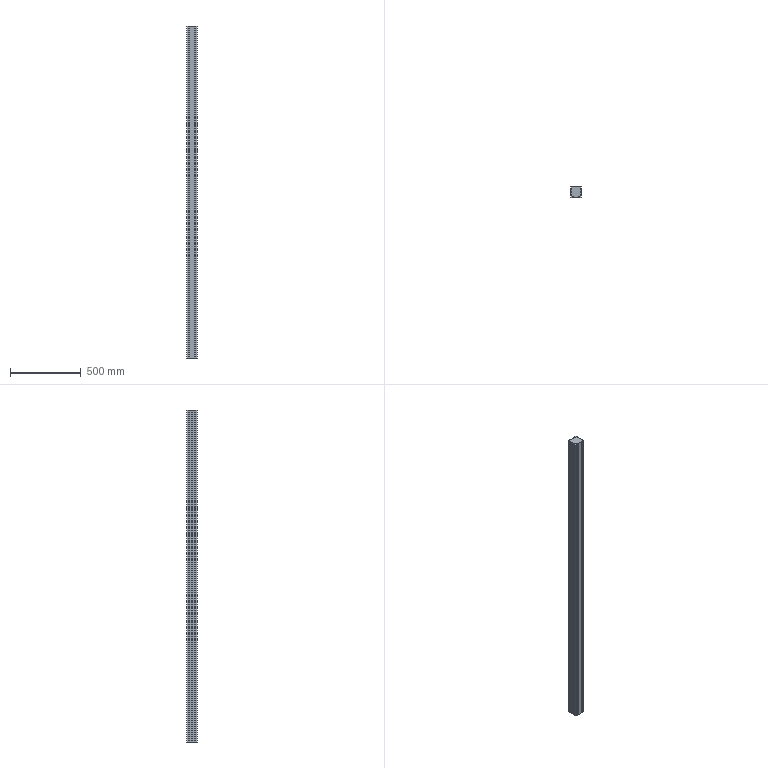Part | SolidWorks | features ICE 3, Extrusion 1, MirrorPattern 1 | 1 solid | 74 faces | box 75 x 75 x 2340 mm | volume 12326933 mm3 | plane 74